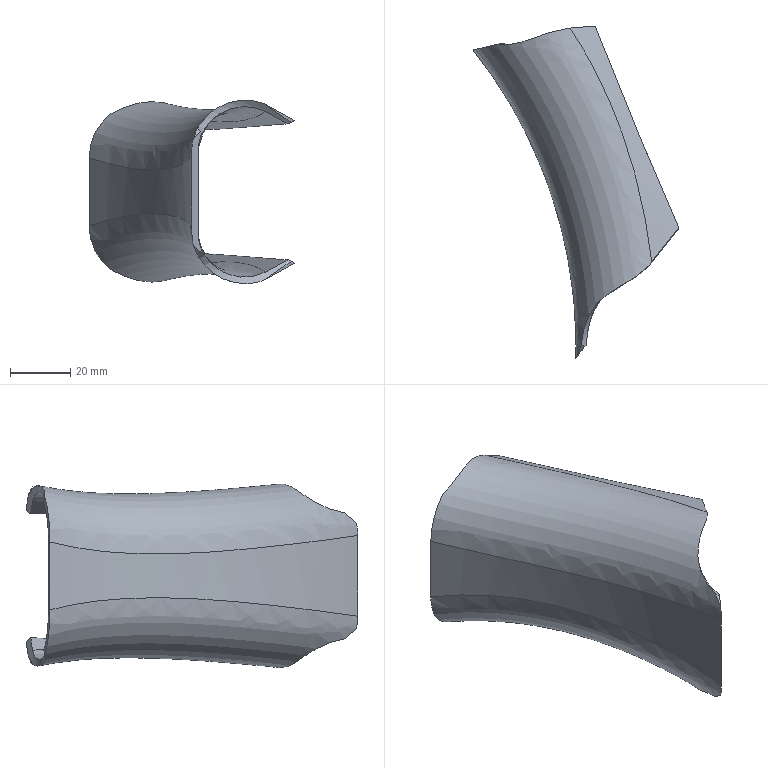Part | STEP file | PRT0001_68_33 | 1 solid | 24 faces | box 68.382 x 110.355 x 61.109 mm | volume 20597 mm3 | spline 10 | cylinder 8 | plane 6 | commonest cylinder face diameters 25 x2 28 x2 50 x2 316.845 x1 320.845 x1